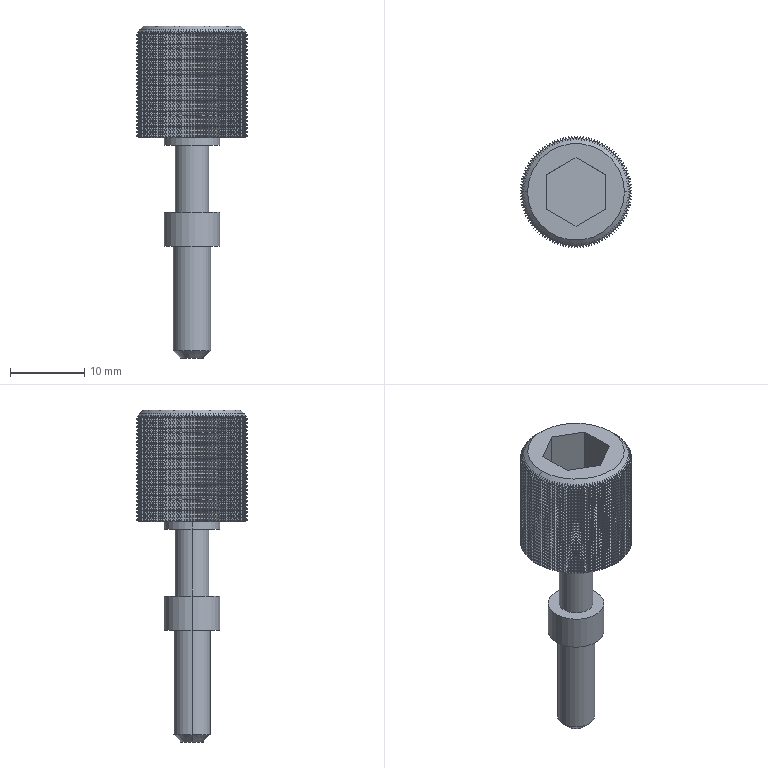Part | SolidWorks | features BaseBody 1 | 1 solid | 13825 faces | volume 2705 mm3 | plane 6973 | cone 6844 | cylinder 8 | commonest cylinder face diameters 7.5 x4 4.5 x2 5 x2